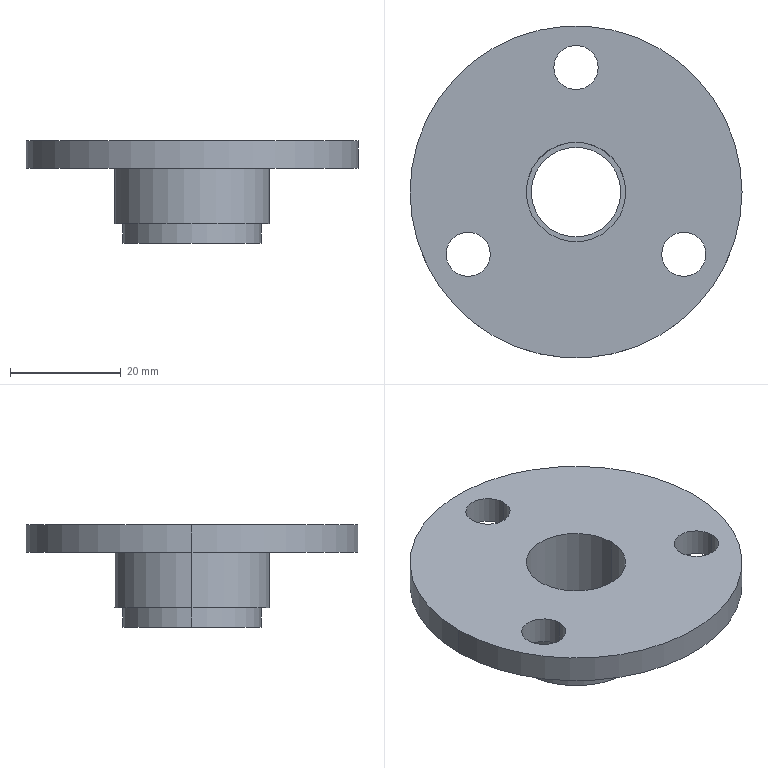Part | SolidWorks | features ICE 2, Extrusion 1 | 1 solid | 21 faces | box 60 x 60 x 18.5 mm | volume 16720 mm3 | cylinder 16 | plane 5 | commonest cylinder face diameters 8 x6 16.2 x2 18 x2 25 x2 28 x2 60 x2
STEP:
#1=CARTESIAN_POINT('',(8.1,0.,-13.5));
#2=VERTEX_POINT('',#1);
#3=CARTESIAN_POINT('',(-8.1,0.,-13.5));
#4=VERTEX_POINT('',#3);
#5=CARTESIAN_POINT('',(0.,0.,-13.5));
#6=DIRECTION('',(0.,0.,-1.));
#7=DIRECTION('',(-1.,0.,0.));
#8=AXIS2_PLACEMENT_3D('',#5,#6,#7);
#9=CIRCLE('',#8,8.1);
#10=EDGE_CURVE('',#2,#4,#9,.T.);
#11=ORIENTED_EDGE('',*,*,#10,.T.);
#12=CARTESIAN_POINT('',(-8.1,0.,-10.));
#13=VERTEX_POINT('',#12);
#14=CARTESIAN_POINT('',(-8.1,0.,-13.5));
#15=DIRECTION('',(0.,0.,1.));
#16=VECTOR('',#15,1000.);
#17=LINE('',#14,#16);
#18=EDGE_CURVE('',#4,#13,#17,.T.);
#19=ORIENTED_EDGE('',*,*,#18,.T.);
#20=CARTESIAN_POINT('',(8.1,0.,-10.));
#21=VERTEX_POINT('',#20);
#22=CARTESIAN_POINT('',(0.,0.,-10.));
#23=DIRECTION('',(0.,0.,-1.));
#24=DIRECTION('',(-1.,0.,0.));
#25=AXIS2_PLACEMENT_3D('',#22,#23,#24);
#26=CIRCLE('',#25,8.1);
#27=EDGE_CURVE('',#21,#13,#26,.T.);
#28=ORIENTED_EDGE('',*,*,#27,.F.);
#29=CARTESIAN_POINT('',(8.1,0.,-13.5));
#30=DIRECTION('',(0.,0.,1.));
#31=VECTOR('',#30,1000.);
#32=LINE('',#29,#31);
#33=EDGE_CURVE('',#2,#21,#32,.T.);
#34=ORIENTED_EDGE('',*,*,#33,.F.);
#35=EDGE_LOOP('',(#11,#19,#28,#34));
#36=FACE_OUTER_BOUND('',#35,.T.);
#37=CARTESIAN_POINT('',(0.,0.,-13.5));
#38=DIRECTION('',(0.,0.,1.));
#39=DIRECTION('',(1.,0.,0.));
#40=AXIS2_PLACEMENT_3D('',#37,#38,#39);
#41=CYLINDRICAL_SURFACE('',#40,8.1);
#42=ADVANCED_FACE('',(#36),#41,.F.);
#43=CARTESIAN_POINT('',(-12.5,0.,-13.5));
#44=VERTEX_POINT('',#43);
#45=CARTESIAN_POINT('',(12.5,0.,-13.5));
#46=VERTEX_POINT('',#45);
#47=CARTESIAN_POINT('',(0.,0.,-13.5));
#48=DIRECTION('',(0.,0.,-1.));
#49=DIRECTION('',(-1.,0.,0.));
#50=AXIS2_PLACEMENT_3D('',#47,#48,#49);
#51=CIRCLE('',#50,12.5);
#52=EDGE_CURVE('',#44,#46,#51,.T.);
#53=ORIENTED_EDGE('',*,*,#52,.F.);
#54=CARTESIAN_POINT('',(-12.5,0.,-10.));
#55=VERTEX_POINT('',#54);
#56=CARTESIAN_POINT('',(-12.5,0.,-13.5));
#57=DIRECTION('',(0.,0.,1.));
#58=VECTOR('',#57,1000.);
#59=LINE('',#56,#58);
#60=EDGE_CURVE('',#44,#55,#59,.T.);
#61=ORIENTED_EDGE('',*,*,#60,.T.);
#62=CARTESIAN_POINT('',(12.5,0.,-10.));
#63=VERTEX_POINT('',#62);
#64=CARTESIAN_POINT('',(0.,0.,-10.));
#65=DIRECTION('',(0.,0.,-1.));
#66=DIRECTION('',(-1.,0.,0.));
#67=AXIS2_PLACEMENT_3D('',#64,#65,#66);
#68=CIRCLE('',#67,12.5);
#69=EDGE_CURVE('',#55,#63,#68,.T.);
#70=ORIENTED_EDGE('',*,*,#69,.T.);
#71=CARTESIAN_POINT('',(12.5,0.,-13.5));
#72=DIRECTION('',(0.,0.,1.));
#73=VECTOR('',#72,1000.);
#74=LINE('',#71,#73);
#75=EDGE_CURVE('',#46,#63,#74,.T.);
#76=ORIENTED_EDGE('',*,*,#75,.F.);
#77=EDGE_LOOP('',(#53,#61,#70,#76));
#78=FACE_OUTER_BOUND('',#77,.T.);
#79=CARTESIAN_POINT('',(0.,0.,-13.5));
#80=DIRECTION('',(0.,0.,1.));
#81=DIRECTION('',(1.,0.,0.));
#82=AXIS2_PLACEMENT_3D('',#79,#80,#81);
#83=CYLINDRICAL_SURFACE('',#82,12.5);
#84=ADVANCED_FACE('',(#78),#83,.T.);
#85=CARTESIAN_POINT('',(-14.,0.,-10.));
#86=VERTEX_POINT('',#85);
#87=CARTESIAN_POINT('',(14.,0.,-10.));
#88=VERTEX_POINT('',#87);
#89=CARTESIAN_POINT('',(0.,0.,-10.));
#90=DIRECTION('',(0.,0.,-1.));
#91=DIRECTION('',(-1.,0.,0.));
#92=AXIS2_PLACEMENT_3D('',#89,#90,#91);
#93=CIRCLE('',#92,14.);
#94=EDGE_CURVE('',#86,#88,#93,.T.);
#95=ORIENTED_EDGE('',*,*,#94,.F.);
#96=CARTESIAN_POINT('',(-14.,0.,0.));
#97=VERTEX_POINT('',#96);
#98=CARTESIAN_POINT('',(-14.,0.,-10.));
#99=DIRECTION('',(0.,0.,1.));
#100=VECTOR('',#99,1000.);
#101=LINE('',#98,#100);
#102=EDGE_CURVE('',#86,#97,#101,.T.);
#103=ORIENTED_EDGE('',*,*,#102,.T.);
#104=CARTESIAN_POINT('',(14.,0.,0.));
#105=VERTEX_POINT('',#104);
#106=CARTESIAN_POINT('',(0.,0.,0.));
#107=DIRECTION('',(0.,0.,-1.));
#108=DIRECTION('',(1.,0.,0.));
#109=AXIS2_PLACEMENT_3D('',#106,#107,#108);
#110=CIRCLE('',#109,14.);
#111=EDGE_CURVE('',#97,#105,#110,.T.);
#112=ORIENTED_EDGE('',*,*,#111,.T.);
#113=CARTESIAN_POINT('',(14.,0.,-10.));
#114=DIRECTION('',(0.,0.,1.));
#115=VECTOR('',#114,1000.);
#116=LINE('',#113,#115);
#117=EDGE_CURVE('',#88,#105,#116,.T.);
#118=ORIENTED_EDGE('',*,*,#117,.F.);
#119=EDGE_LOOP('',(#95,#103,#112,#118));
#120=FACE_OUTER_BOUND('',#119,.T.);
#121=CARTESIAN_POINT('',(0.,0.,-10.));
#122=DIRECTION('',(0.,0.,1.));
#123=DIRECTION('',(1.,0.,0.));
#124=AXIS2_PLACEMENT_3D('',#121,#122,#123);
#125=CYLINDRICAL_SURFACE('',#124,14.);
#126=ADVANCED_FACE('',(#120),#125,.T.);
#127=CARTESIAN_POINT('',(-23.486,-11.25,5.));
#128=VERTEX_POINT('',#127);
#129=CARTESIAN_POINT('',(-15.486,-11.25,5.));
#130=VERTEX_POINT('',#129);
#131=CARTESIAN_POINT('',(-19.486,-11.25,5.));
#132=DIRECTION('',(0.,0.,1.));
#133=DIRECTION('',(1.,0.,0.));
#134=AXIS2_PLACEMENT_3D('',#131,#132,#133);
#135=CIRCLE('',#134,4.);
#136=EDGE_CURVE('',#128,#130,#135,.T.);
#137=ORIENTED_EDGE('',*,*,#136,.T.);
#138=CARTESIAN_POINT('',(-15.486,-11.25,0.));
#139=VERTEX_POINT('',#138);
#140=CARTESIAN_POINT('',(-15.486,-11.25,5.));
#141=DIRECTION('',(0.,0.,-1.));
#142=VECTOR('',#141,1000.);
#143=LINE('',#140,#142);
#144=EDGE_CURVE('',#130,#139,#143,.T.);
#145=ORIENTED_EDGE('',*,*,#144,.T.);
#146=CARTESIAN_POINT('',(-23.486,-11.25,0.));
#147=VERTEX_POINT('',#146);
#148=CARTESIAN_POINT('',(-19.486,-11.25,0.));
#149=DIRECTION('',(0.,0.,1.));
#150=DIRECTION('',(1.,0.,0.));
#151=AXIS2_PLACEMENT_3D('',#148,#149,#150);
#152=CIRCLE('',#151,4.);
#153=EDGE_CURVE('',#147,#139,#152,.T.);
#154=ORIENTED_EDGE('',*,*,#153,.F.);
#155=CARTESIAN_POINT('',(-23.486,-11.25,5.));
#156=DIRECTION('',(0.,0.,-1.));
#157=VECTOR('',#156,1000.);
#158=LINE('',#155,#157);
#159=EDGE_CURVE('',#128,#147,#158,.T.);
#160=ORIENTED_EDGE('',*,*,#159,.F.);
#161=EDGE_LOOP('',(#137,#145,#154,#160));
#162=FACE_OUTER_BOUND('',#161,.T.);
#163=CARTESIAN_POINT('',(-19.486,-11.25,5.));
#164=DIRECTION('',(0.,0.,-1.));
#165=DIRECTION('',(-1.,0.,0.));
#166=AXIS2_PLACEMENT_3D('',#163,#164,#165);
#167=CYLINDRICAL_SURFACE('',#166,4.);
#168=ADVANCED_FACE('',(#162),#167,.F.);
#169=CARTESIAN_POINT('',(15.486,-11.25,5.));
#170=VERTEX_POINT('',#169);
#171=CARTESIAN_POINT('',(23.486,-11.25,5.));
#172=VERTEX_POINT('',#171);
#173=CARTESIAN_POINT('',(19.486,-11.25,5.));
#174=DIRECTION('',(0.,0.,1.));
#175=DIRECTION('',(1.,0.,0.));
#176=AXIS2_PLACEMENT_3D('',#173,#174,#175);
#177=CIRCLE('',#176,4.);
#178=EDGE_CURVE('',#170,#172,#177,.T.);
#179=ORIENTED_EDGE('',*,*,#178,.T.);
#180=CARTESIAN_POINT('',(23.486,-11.25,0.));
#181=VERTEX_POINT('',#180);
#182=CARTESIAN_POINT('',(23.486,-11.25,5.));
#183=DIRECTION('',(0.,0.,-1.));
#184=VECTOR('',#183,1000.);
#185=LINE('',#182,#184);
#186=EDGE_CURVE('',#172,#181,#185,.T.);
#187=ORIENTED_EDGE('',*,*,#186,.T.);
#188=CARTESIAN_POINT('',(15.486,-11.25,0.));
#189=VERTEX_POINT('',#188);
#190=CARTESIAN_POINT('',(19.486,-11.25,0.));
#191=DIRECTION('',(0.,0.,1.));
#192=DIRECTION('',(1.,0.,0.));
#193=AXIS2_PLACEMENT_3D('',#190,#191,#192);
#194=CIRCLE('',#193,4.);
#195=EDGE_CURVE('',#189,#181,#194,.T.);
#196=ORIENTED_EDGE('',*,*,#195,.F.);
#197=CARTESIAN_POINT('',(15.486,-11.25,5.));
#198=DIRECTION('',(0.,0.,-1.));
#199=VECTOR('',#198,1000.);
#200=LINE('',#197,#199);
#201=EDGE_CURVE('',#170,#189,#200,.T.);
#202=ORIENTED_EDGE('',*,*,#201,.F.);
#203=EDGE_LOOP('',(#179,#187,#196,#202));
#204=FACE_OUTER_BOUND('',#203,.T.);
#205=CARTESIAN_POINT('',(19.486,-11.25,5.));
#206=DIRECTION('',(0.,0.,-1.));
#207=DIRECTION('',(-1.,0.,0.));
#208=AXIS2_PLACEMENT_3D('',#205,#206,#207);
#209=CYLINDRICAL_SURFACE('',#208,4.);
#210=ADVANCED_FACE('',(#204),#209,.F.);
#211=CARTESIAN_POINT('',(-4.,22.5,5.));
#212=VERTEX_POINT('',#211);
#213=CARTESIAN_POINT('',(4.,22.5,5.));
#214=VERTEX_POINT('',#213);
#215=CARTESIAN_POINT('',(0.,22.5,5.));
#216=DIRECTION('',(0.,0.,1.));
#217=DIRECTION('',(1.,0.,0.));
#218=AXIS2_PLACEMENT_3D('',#215,#216,#217);
#219=CIRCLE('',#218,4.);
#220=EDGE_CURVE('',#212,#214,#219,.T.);
#221=ORIENTED_EDGE('',*,*,#220,.T.);
#222=CARTESIAN_POINT('',(4.,22.5,0.));
#223=VERTEX_POINT('',#222);
#224=CARTESIAN_POINT('',(4.,22.5,5.));
#225=DIRECTION('',(0.,0.,-1.));
#226=VECTOR('',#225,1000.);
#227=LINE('',#224,#226);
#228=EDGE_CURVE('',#214,#223,#227,.T.);
#229=ORIENTED_EDGE('',*,*,#228,.T.);
#230=CARTESIAN_POINT('',(-4.,22.5,0.));
#231=VERTEX_POINT('',#230);
#232=CARTESIAN_POINT('',(0.,22.5,0.));
#233=DIRECTION('',(0.,0.,1.));
#234=DIRECTION('',(1.,0.,0.));
#235=AXIS2_PLACEMENT_3D('',#232,#233,#234);
#236=CIRCLE('',#235,4.);
#237=EDGE_CURVE('',#231,#223,#236,.T.);
#238=ORIENTED_EDGE('',*,*,#237,.F.);
#239=CARTESIAN_POINT('',(-4.,22.5,5.));
#240=DIRECTION('',(0.,0.,-1.));
#241=VECTOR('',#240,1000.);
#242=LINE('',#239,#241);
#243=EDGE_CURVE('',#212,#231,#242,.T.);
#244=ORIENTED_EDGE('',*,*,#243,.F.);
#245=EDGE_LOOP('',(#221,#229,#238,#244));
#246=FACE_OUTER_BOUND('',#245,.T.);
#247=CARTESIAN_POINT('',(0.,22.5,5.));
#248=DIRECTION('',(0.,0.,-1.));
#249=DIRECTION('',(-1.,0.,0.));
#250=AXIS2_PLACEMENT_3D('',#247,#248,#249);
#251=CYLINDRICAL_SURFACE('',#250,4.);
#252=ADVANCED_FACE('',(#246),#251,.F.);
#253=CARTESIAN_POINT('',(-9.,0.,5.));
#254=VERTEX_POINT('',#253);
#255=CARTESIAN_POINT('',(9.,0.,5.));
#256=VERTEX_POINT('',#255);
#257=CARTESIAN_POINT('',(0.,0.,5.));
#258=DIRECTION('',(0.,0.,1.));
#259=DIRECTION('',(1.,0.,0.));
#260=AXIS2_PLACEMENT_3D('',#257,#258,#259);
#261=CIRCLE('',#260,9.);
#262=EDGE_CURVE('',#254,#256,#261,.T.);
#263=ORIENTED_EDGE('',*,*,#262,.T.);
#264=CARTESIAN_POINT('',(9.,0.,-10.));
#265=VERTEX_POINT('',#264);
#266=CARTESIAN_POINT('',(9.,0.,5.));
#267=DIRECTION('',(0.,0.,-1.));
#268=VECTOR('',#267,1000.);
#269=LINE('',#266,#268);
#270=EDGE_CURVE('',#256,#265,#269,.T.);
#271=ORIENTED_EDGE('',*,*,#270,.T.);
#272=CARTESIAN_POINT('',(-9.,0.,-10.));
#273=VERTEX_POINT('',#272);
#274=CARTESIAN_POINT('',(0.,0.,-10.));
#275=DIRECTION('',(0.,0.,-1.));
#276=DIRECTION('',(-1.,0.,0.));
#277=AXIS2_PLACEMENT_3D('',#274,#275,#276);
#278=CIRCLE('',#277,9.);
#279=EDGE_CURVE('',#265,#273,#278,.T.);
#280=ORIENTED_EDGE('',*,*,#279,.T.);
#281=CARTESIAN_POINT('',(-9.,0.,5.));
#282=DIRECTION('',(0.,0.,-1.));
#283=VECTOR('',#282,1000.);
#284=LINE('',#281,#283);
#285=EDGE_CURVE('',#254,#273,#284,.T.);
#286=ORIENTED_EDGE('',*,*,#285,.F.);
#287=EDGE_LOOP('',(#263,#271,#280,#286));
#288=FACE_OUTER_BOUND('',#287,.T.);
#289=CARTESIAN_POINT('',(0.,0.,5.));
#290=DIRECTION('',(0.,0.,-1.));
#291=DIRECTION('',(-1.,0.,0.));
#292=AXIS2_PLACEMENT_3D('',#289,#290,#291);
#293=CYLINDRICAL_SURFACE('',#292,9.);
#294=ADVANCED_FACE('',(#288),#293,.F.);
#295=CARTESIAN_POINT('',(30.,0.,5.));
#296=VERTEX_POINT('',#295);
#297=CARTESIAN_POINT('',(-30.,0.,5.));
#298=VERTEX_POINT('',#297);
#299=CARTESIAN_POINT('',(0.,0.,5.));
#300=DIRECTION('',(0.,0.,1.));
#301=DIRECTION('',(1.,0.,0.));
#302=AXIS2_PLACEMENT_3D('',#299,#300,#301);
#303=CIRCLE('',#302,30.);
#304=EDGE_CURVE('',#296,#298,#303,.T.);
#305=ORIENTED_EDGE('',*,*,#304,.F.);
#306=CARTESIAN_POINT('',(30.,0.,0.));
#307=VERTEX_POINT('',#306);
#308=CARTESIAN_POINT('',(30.,0.,5.));
#309=DIRECTION('',(0.,0.,-1.));
#310=VECTOR('',#309,1000.);
#311=LINE('',#308,#310);
#312=EDGE_CURVE('',#296,#307,#311,.T.);
#313=ORIENTED_EDGE('',*,*,#312,.T.);
#314=CARTESIAN_POINT('',(-30.,0.,0.));
#315=VERTEX_POINT('',#314);
#316=CARTESIAN_POINT('',(0.,0.,0.));
#317=DIRECTION('',(0.,0.,1.));
#318=DIRECTION('',(1.,0.,0.));
#319=AXIS2_PLACEMENT_3D('',#316,#317,#318);
#320=CIRCLE('',#319,30.);
#321=EDGE_CURVE('',#307,#315,#320,.T.);
#322=ORIENTED_EDGE('',*,*,#321,.T.);
#323=CARTESIAN_POINT('',(-30.,0.,5.));
#324=DIRECTION('',(0.,0.,-1.));
#325=VECTOR('',#324,1000.);
#326=LINE('',#323,#325);
#327=EDGE_CURVE('',#298,#315,#326,.T.);
#328=ORIENTED_EDGE('',*,*,#327,.F.);
#329=EDGE_LOOP('',(#305,#313,#322,#328));
#330=FACE_OUTER_BOUND('',#329,.T.);
#331=CARTESIAN_POINT('',(0.,0.,5.));
#332=DIRECTION('',(0.,0.,-1.));
#333=DIRECTION('',(-1.,0.,0.));
#334=AXIS2_PLACEMENT_3D('',#331,#332,#333);
#335=CYLINDRICAL_SURFACE('',#334,30.);
#336=ADVANCED_FACE('',(#330),#335,.T.);
#337=ORIENTED_EDGE('',*,*,#153,.T.);
#338=CARTESIAN_POINT('',(-19.486,-11.25,0.));
#339=DIRECTION('',(0.,0.,1.));
#340=DIRECTION('',(1.,0.,0.));
#341=AXIS2_PLACEMENT_3D('',#338,#339,#340);
#342=CIRCLE('',#341,4.);
#343=EDGE_CURVE('',#139,#147,#342,.T.);
#344=ORIENTED_EDGE('',*,*,#343,.T.);
#345=EDGE_LOOP('',(#337,#344));
#346=FACE_BOUND('',#345,.T.);
#347=ORIENTED_EDGE('',*,*,#195,.T.);
#348=CARTESIAN_POINT('',(19.486,-11.25,0.));
#349=DIRECTION('',(0.,0.,1.));
#350=DIRECTION('',(1.,0.,0.));
#351=AXIS2_PLACEMENT_3D('',#348,#349,#350);
#352=CIRCLE('',#351,4.);
#353=EDGE_CURVE('',#181,#189,#352,.T.);
#354=ORIENTED_EDGE('',*,*,#353,.T.);
#355=EDGE_LOOP('',(#347,#354));
#356=FACE_BOUND('',#355,.T.);
#357=ORIENTED_EDGE('',*,*,#237,.T.);
#358=CARTESIAN_POINT('',(0.,22.5,0.));
#359=DIRECTION('',(0.,0.,1.));
#360=DIRECTION('',(1.,0.,0.));
#361=AXIS2_PLACEMENT_3D('',#358,#359,#360);
#362=CIRCLE('',#361,4.);
#363=EDGE_CURVE('',#223,#231,#362,.T.);
#364=ORIENTED_EDGE('',*,*,#363,.T.);
#365=EDGE_LOOP('',(#357,#364));
#366=FACE_BOUND('',#365,.T.);
#367=CARTESIAN_POINT('',(0.,0.,0.));
#368=DIRECTION('',(0.,0.,1.));
#369=DIRECTION('',(1.,0.,0.));
#370=AXIS2_PLACEMENT_3D('',#367,#368,#369);
#371=CIRCLE('',#370,30.);
#372=EDGE_CURVE('',#315,#307,#371,.T.);
#373=ORIENTED_EDGE('',*,*,#372,.F.);
#374=ORIENTED_EDGE('',*,*,#321,.F.);
#375=EDGE_LOOP('',(#373,#374));
#376=FACE_OUTER_BOUND('',#375,.T.);
#377=CARTESIAN_POINT('',(0.,0.,0.));
#378=DIRECTION('',(0.,0.,-1.));
#379=DIRECTION('',(1.,0.,0.));
#380=AXIS2_PLACEMENT_3D('',#377,#378,#379);
#381=CIRCLE('',#380,14.);
#382=EDGE_CURVE('',#105,#97,#381,.T.);
#383=ORIENTED_EDGE('',*,*,#382,.F.);
#384=ORIENTED_EDGE('',*,*,#111,.F.);
#385=EDGE_LOOP('',(#383,#384));
#386=FACE_BOUND('',#385,.T.);
#387=CARTESIAN_POINT('',(0.,0.,0.));
#388=DIRECTION('',(0.,0.,1.));
#389=DIRECTION('',(1.,0.,0.));
#390=AXIS2_PLACEMENT_3D('',#387,#388,#389);
#391=PLANE('',#390);
#392=ADVANCED_FACE('',(#346,#356,#366,#376,#386),#391,.F.);
#393=ORIENTED_EDGE('',*,*,#178,.F.);
#394=CARTESIAN_POINT('',(19.486,-11.25,5.));
#395=DIRECTION('',(0.,0.,1.));
#396=DIRECTION('',(1.,0.,0.));
#397=AXIS2_PLACEMENT_3D('',#394,#395,#396);
#398=CIRCLE('',#397,4.);
#399=EDGE_CURVE('',#172,#170,#398,.T.);
#400=ORIENTED_EDGE('',*,*,#399,.F.);
#401=EDGE_LOOP('',(#393,#400));
#402=FACE_BOUND('',#401,.T.);
#403=ORIENTED_EDGE('',*,*,#262,.F.);
#404=CARTESIAN_POINT('',(0.,0.,5.));
#405=DIRECTION('',(0.,0.,1.));
#406=DIRECTION('',(1.,0.,0.));
#407=AXIS2_PLACEMENT_3D('',#404,#405,#406);
#408=CIRCLE('',#407,9.);
#409=EDGE_CURVE('',#256,#254,#408,.T.);
#410=ORIENTED_EDGE('',*,*,#409,.F.);
#411=EDGE_LOOP('',(#403,#410));
#412=FACE_BOUND('',#411,.T.);
#413=CARTESIAN_POINT('',(0.,0.,5.));
#414=DIRECTION('',(0.,0.,1.));
#415=DIRECTION('',(1.,0.,0.));
#416=AXIS2_PLACEMENT_3D('',#413,#414,#415);
#417=CIRCLE('',#416,30.);
#418=EDGE_CURVE('',#298,#296,#417,.T.);
#419=ORIENTED_EDGE('',*,*,#418,.T.);
#420=ORIENTED_EDGE('',*,*,#304,.T.);
#421=EDGE_LOOP('',(#419,#420));
#422=FACE_OUTER_BOUND('',#421,.T.);
#423=ORIENTED_EDGE('',*,*,#220,.F.);
#424=CARTESIAN_POINT('',(0.,22.5,5.));
#425=DIRECTION('',(0.,0.,1.));
#426=DIRECTION('',(1.,0.,0.));
#427=AXIS2_PLACEMENT_3D('',#424,#425,#426);
#428=CIRCLE('',#427,4.);
#429=EDGE_CURVE('',#214,#212,#428,.T.);
#430=ORIENTED_EDGE('',*,*,#429,.F.);
#431=EDGE_LOOP('',(#423,#430));
#432=FACE_BOUND('',#431,.T.);
#433=ORIENTED_EDGE('',*,*,#136,.F.);
#434=CARTESIAN_POINT('',(-19.486,-11.25,5.));
#435=DIRECTION('',(0.,0.,1.));
#436=DIRECTION('',(1.,0.,0.));
#437=AXIS2_PLACEMENT_3D('',#434,#435,#436);
#438=CIRCLE('',#437,4.);
#439=EDGE_CURVE('',#130,#128,#438,.T.);
#440=ORIENTED_EDGE('',*,*,#439,.F.);
#441=EDGE_LOOP('',(#433,#440));
#442=FACE_BOUND('',#441,.T.);
#443=CARTESIAN_POINT('',(0.,0.,5.));
#444=DIRECTION('',(0.,0.,1.));
#445=DIRECTION('',(1.,0.,0.));
#446=AXIS2_PLACEMENT_3D('',#443,#444,#445);
#447=PLANE('',#446);
#448=ADVANCED_FACE('',(#402,#412,#422,#432,#442),#447,.T.);
#449=ORIENTED_EDGE('',*,*,#312,.F.);
#450=ORIENTED_EDGE('',*,*,#418,.F.);
#451=ORIENTED_EDGE('',*,*,#327,.T.);
#452=ORIENTED_EDGE('',*,*,#372,.T.);
#453=EDGE_LOOP('',(#449,#450,#451,#452));
#454=FACE_OUTER_BOUND('',#453,.T.);
#455=CARTESIAN_POINT('',(0.,0.,5.));
#456=DIRECTION('',(0.,0.,-1.));
#457=DIRECTION('',(-1.,0.,0.));
#458=AXIS2_PLACEMENT_3D('',#455,#456,#457);
#459=CYLINDRICAL_SURFACE('',#458,30.);
#460=ADVANCED_FACE('',(#454),#459,.T.);
#461=ORIENTED_EDGE('',*,*,#270,.F.);
#462=ORIENTED_EDGE('',*,*,#409,.T.);
#463=ORIENTED_EDGE('',*,*,#285,.T.);
#464=CARTESIAN_POINT('',(0.,0.,-10.));
#465=DIRECTION('',(0.,0.,-1.));
#466=DIRECTION('',(-1.,0.,0.));
#467=AXIS2_PLACEMENT_3D('',#464,#465,#466);
#468=CIRCLE('',#467,9.);
#469=EDGE_CURVE('',#273,#265,#468,.T.);
#470=ORIENTED_EDGE('',*,*,#469,.T.);
#471=EDGE_LOOP('',(#461,#462,#463,#470));
#472=FACE_OUTER_BOUND('',#471,.T.);
#473=CARTESIAN_POINT('',(0.,0.,5.));
#474=DIRECTION('',(0.,0.,-1.));
#475=DIRECTION('',(-1.,0.,0.));
#476=AXIS2_PLACEMENT_3D('',#473,#474,#475);
#477=CYLINDRICAL_SURFACE('',#476,9.);
#478=ADVANCED_FACE('',(#472),#477,.F.);
#479=ORIENTED_EDGE('',*,*,#228,.F.);
#480=ORIENTED_EDGE('',*,*,#429,.T.);
#481=ORIENTED_EDGE('',*,*,#243,.T.);
#482=ORIENTED_EDGE('',*,*,#363,.F.);
#483=EDGE_LOOP('',(#479,#480,#481,#482));
#484=FACE_OUTER_BOUND('',#483,.T.);
#485=CARTESIAN_POINT('',(0.,22.5,5.));
#486=DIRECTION('',(0.,0.,-1.));
#487=DIRECTION('',(-1.,0.,0.));
#488=AXIS2_PLACEMENT_3D('',#485,#486,#487);
#489=CYLINDRICAL_SURFACE('',#488,4.);
#490=ADVANCED_FACE('',(#484),#489,.F.);
#491=ORIENTED_EDGE('',*,*,#186,.F.);
#492=ORIENTED_EDGE('',*,*,#399,.T.);
#493=ORIENTED_EDGE('',*,*,#201,.T.);
#494=ORIENTED_EDGE('',*,*,#353,.F.);
#495=EDGE_LOOP('',(#491,#492,#493,#494));
#496=FACE_OUTER_BOUND('',#495,.T.);
#497=CARTESIAN_POINT('',(19.486,-11.25,5.));
#498=DIRECTION('',(0.,0.,-1.));
#499=DIRECTION('',(-1.,0.,0.));
#500=AXIS2_PLACEMENT_3D('',#497,#498,#499);
#501=CYLINDRICAL_SURFACE('',#500,4.);
#502=ADVANCED_FACE('',(#496),#501,.F.);
#503=ORIENTED_EDGE('',*,*,#144,.F.);
#504=ORIENTED_EDGE('',*,*,#439,.T.);
#505=ORIENTED_EDGE('',*,*,#159,.T.);
#506=ORIENTED_EDGE('',*,*,#343,.F.);
#507=EDGE_LOOP('',(#503,#504,#505,#506));
#508=FACE_OUTER_BOUND('',#507,.T.);
#509=CARTESIAN_POINT('',(-19.486,-11.25,5.));
#510=DIRECTION('',(0.,0.,-1.));
#511=DIRECTION('',(-1.,0.,0.));
#512=AXIS2_PLACEMENT_3D('',#509,#510,#511);
#513=CYLINDRICAL_SURFACE('',#512,4.);
#514=ADVANCED_FACE('',(#508),#513,.F.);
#515=CARTESIAN_POINT('',(0.,0.,-10.));
#516=DIRECTION('',(0.,0.,-1.));
#517=DIRECTION('',(-1.,0.,0.));
#518=AXIS2_PLACEMENT_3D('',#515,#516,#517);
#519=CIRCLE('',#518,12.5);
#520=EDGE_CURVE('',#63,#55,#519,.T.);
#521=ORIENTED_EDGE('',*,*,#520,.F.);
#522=ORIENTED_EDGE('',*,*,#69,.F.);
#523=EDGE_LOOP('',(#521,#522));
#524=FACE_BOUND('',#523,.T.);
#525=CARTESIAN_POINT('',(0.,0.,-10.));
#526=DIRECTION('',(0.,0.,-1.));
#527=DIRECTION('',(-1.,0.,0.));
#528=AXIS2_PLACEMENT_3D('',#525,#526,#527);
#529=CIRCLE('',#528,14.);
#530=EDGE_CURVE('',#88,#86,#529,.T.);
#531=ORIENTED_EDGE('',*,*,#530,.T.);
#532=ORIENTED_EDGE('',*,*,#94,.T.);
#533=EDGE_LOOP('',(#531,#532));
#534=FACE_OUTER_BOUND('',#533,.T.);
#535=CARTESIAN_POINT('',(0.,0.,-10.));
#536=DIRECTION('',(0.,0.,-1.));
#537=DIRECTION('',(-1.,0.,0.));
#538=AXIS2_PLACEMENT_3D('',#535,#536,#537);
#539=PLANE('',#538);
#540=ADVANCED_FACE('',(#524,#534),#539,.T.);
#541=ORIENTED_EDGE('',*,*,#102,.F.);
#542=ORIENTED_EDGE('',*,*,#530,.F.);
#543=ORIENTED_EDGE('',*,*,#117,.T.);
#544=ORIENTED_EDGE('',*,*,#382,.T.);
#545=EDGE_LOOP('',(#541,#542,#543,#544));
#546=FACE_OUTER_BOUND('',#545,.T.);
#547=CARTESIAN_POINT('',(0.,0.,-10.));
#548=DIRECTION('',(0.,0.,1.));
#549=DIRECTION('',(1.,0.,0.));
#550=AXIS2_PLACEMENT_3D('',#547,#548,#549);
#551=CYLINDRICAL_SURFACE('',#550,14.);
#552=ADVANCED_FACE('',(#546),#551,.T.);
#553=CARTESIAN_POINT('',(0.,0.,-13.5));
#554=DIRECTION('',(0.,0.,-1.));
#555=DIRECTION('',(-1.,0.,0.));
#556=AXIS2_PLACEMENT_3D('',#553,#554,#555);
#557=CIRCLE('',#556,12.5);
#558=EDGE_CURVE('',#46,#44,#557,.T.);
#559=ORIENTED_EDGE('',*,*,#558,.T.);
#560=ORIENTED_EDGE('',*,*,#52,.T.);
#561=EDGE_LOOP('',(#559,#560));
#562=FACE_OUTER_BOUND('',#561,.T.);
#563=ORIENTED_EDGE('',*,*,#10,.F.);
#564=CARTESIAN_POINT('',(0.,0.,-13.5));
#565=DIRECTION('',(0.,0.,-1.));
#566=DIRECTION('',(-1.,0.,0.));
#567=AXIS2_PLACEMENT_3D('',#564,#565,#566);
#568=CIRCLE('',#567,8.1);
#569=EDGE_CURVE('',#4,#2,#568,.T.);
#570=ORIENTED_EDGE('',*,*,#569,.F.);
#571=EDGE_LOOP('',(#563,#570));
#572=FACE_BOUND('',#571,.T.);
#573=CARTESIAN_POINT('',(0.,0.,-13.5));
#574=DIRECTION('',(0.,0.,-1.));
#575=DIRECTION('',(-1.,0.,0.));
#576=AXIS2_PLACEMENT_3D('',#573,#574,#575);
#577=PLANE('',#576);
#578=ADVANCED_FACE('',(#562,#572),#577,.T.);
#579=ORIENTED_EDGE('',*,*,#469,.F.);
#580=ORIENTED_EDGE('',*,*,#279,.F.);
#581=EDGE_LOOP('',(#579,#580));
#582=FACE_OUTER_BOUND('',#581,.T.);
#583=ORIENTED_EDGE('',*,*,#27,.T.);
#584=CARTESIAN_POINT('',(0.,0.,-10.));
#585=DIRECTION('',(0.,0.,-1.));
#586=DIRECTION('',(-1.,0.,0.));
#587=AXIS2_PLACEMENT_3D('',#584,#585,#586);
#588=CIRCLE('',#587,8.1);
#589=EDGE_CURVE('',#13,#21,#588,.T.);
#590=ORIENTED_EDGE('',*,*,#589,.T.);
#591=EDGE_LOOP('',(#583,#590));
#592=FACE_BOUND('',#591,.T.);
#593=CARTESIAN_POINT('',(0.,0.,-10.));
#594=DIRECTION('',(0.,0.,-1.));
#595=DIRECTION('',(-1.,0.,0.));
#596=AXIS2_PLACEMENT_3D('',#593,#594,#595);
#597=PLANE('',#596);
#598=ADVANCED_FACE('',(#582,#592),#597,.F.);
#599=ORIENTED_EDGE('',*,*,#60,.F.);
#600=ORIENTED_EDGE('',*,*,#558,.F.);
#601=ORIENTED_EDGE('',*,*,#75,.T.);
#602=ORIENTED_EDGE('',*,*,#520,.T.);
#603=EDGE_LOOP('',(#599,#600,#601,#602));
#604=FACE_OUTER_BOUND('',#603,.T.);
#605=CARTESIAN_POINT('',(0.,0.,-13.5));
#606=DIRECTION('',(0.,0.,1.));
#607=DIRECTION('',(1.,0.,0.));
#608=AXIS2_PLACEMENT_3D('',#605,#606,#607);
#609=CYLINDRICAL_SURFACE('',#608,12.5);
#610=ADVANCED_FACE('',(#604),#609,.T.);
#611=ORIENTED_EDGE('',*,*,#18,.F.);
#612=ORIENTED_EDGE('',*,*,#569,.T.);
#613=ORIENTED_EDGE('',*,*,#33,.T.);
#614=ORIENTED_EDGE('',*,*,#589,.F.);
#615=EDGE_LOOP('',(#611,#612,#613,#614));
#616=FACE_OUTER_BOUND('',#615,.T.);
#617=CARTESIAN_POINT('',(0.,0.,-13.5));
#618=DIRECTION('',(0.,0.,1.));
#619=DIRECTION('',(1.,0.,0.));
#620=AXIS2_PLACEMENT_3D('',#617,#618,#619);
#621=CYLINDRICAL_SURFACE('',#620,8.1);
#622=ADVANCED_FACE('',(#616),#621,.F.);
#623=CLOSED_SHELL('',(#42,#84,#126,#168,#210,#252,#294,#336,#392,#448,#460,#478,#490,#502,#514,#540,#552,#578,#598,#610,#622));
#624=MANIFOLD_SOLID_BREP('',#623);
#625=CARTESIAN_POINT('',(0.,0.,0.));
#626=DIRECTION('',(0.,0.,1.));
#627=DIRECTION('',(1.,0.,0.));
#628=AXIS2_PLACEMENT_3D('',#625,#626,#627);
#629=(LENGTH_UNIT()NAMED_UNIT(*)SI_UNIT(.MILLI.,.METRE.));
#630=UNCERTAINTY_MEASURE_WITH_UNIT(LENGTH_MEASURE(0.00001),#629,'','');
#631=(NAMED_UNIT(*)PLANE_ANGLE_UNIT()SI_UNIT($,.RADIAN.));
#632=(NAMED_UNIT(*)SI_UNIT($,.STERADIAN.)SOLID_ANGLE_UNIT());
#633=(GEOMETRIC_REPRESENTATION_CONTEXT(3)GLOBAL_UNCERTAINTY_ASSIGNED_CONTEXT((#630))GLOBAL_UNIT_ASSIGNED_CONTEXT((#629,#631,#632))REPRESENTATION_CONTEXT('',''));
#634=ADVANCED_BREP_SHAPE_REPRESENTATION('',(#624,#628),#633);